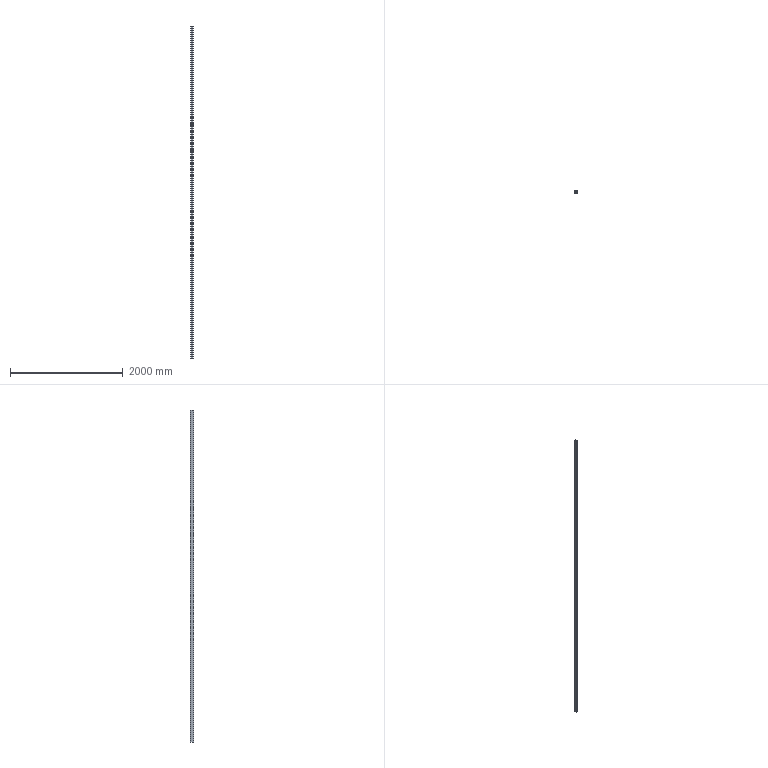Part | SolidWorks | features Extrusion 1 | 1 solid | 18 faces | box 40 x 60 x 5880 mm | volume 2698361 mm3 | plane 10 | cylinder 8 | commonest cylinder face diameters 5 x4 10 x4
STEP:
#1=CARTESIAN_POINT('',(35.,0.,5880.));
#2=VERTEX_POINT('',#1);
#3=CARTESIAN_POINT('',(40.,5.,5880.));
#4=VERTEX_POINT('',#3);
#5=CARTESIAN_POINT('',(35.,5.,5880.));
#6=DIRECTION('',(0.,0.,1.));
#7=DIRECTION('',(-1.,0.,0.));
#8=AXIS2_PLACEMENT_3D('',#5,#6,#7);
#9=CIRCLE('',#8,5.);
#10=EDGE_CURVE('',#2,#4,#9,.T.);
#11=ORIENTED_EDGE('',*,*,#10,.T.);
#12=CARTESIAN_POINT('',(40.,55.,5880.));
#13=VERTEX_POINT('',#12);
#14=CARTESIAN_POINT('',(40.,5.,5880.));
#15=DIRECTION('',(0.,1.,0.));
#16=VECTOR('',#15,1000.);
#17=LINE('',#14,#16);
#18=EDGE_CURVE('',#4,#13,#17,.T.);
#19=ORIENTED_EDGE('',*,*,#18,.T.);
#20=CARTESIAN_POINT('',(35.,60.,5880.));
#21=VERTEX_POINT('',#20);
#22=CARTESIAN_POINT('',(35.,55.,5880.));
#23=DIRECTION('',(0.,0.,1.));
#24=DIRECTION('',(1.,0.,0.));
#25=AXIS2_PLACEMENT_3D('',#22,#23,#24);
#26=CIRCLE('',#25,5.);
#27=EDGE_CURVE('',#13,#21,#26,.T.);
#28=ORIENTED_EDGE('',*,*,#27,.T.);
#29=CARTESIAN_POINT('',(5.,60.,5880.));
#30=VERTEX_POINT('',#29);
#31=CARTESIAN_POINT('',(5.,60.,5880.));
#32=DIRECTION('',(-1.,0.,0.));
#33=VECTOR('',#32,1000.);
#34=LINE('',#31,#33);
#35=EDGE_CURVE('',#21,#30,#34,.T.);
#36=ORIENTED_EDGE('',*,*,#35,.T.);
#37=CARTESIAN_POINT('',(0.,55.,5880.));
#38=VERTEX_POINT('',#37);
#39=CARTESIAN_POINT('',(5.,55.,5880.));
#40=DIRECTION('',(0.,0.,1.));
#41=DIRECTION('',(-1.,0.,0.));
#42=AXIS2_PLACEMENT_3D('',#39,#40,#41);
#43=CIRCLE('',#42,5.);
#44=EDGE_CURVE('',#30,#38,#43,.T.);
#45=ORIENTED_EDGE('',*,*,#44,.T.);
#46=CARTESIAN_POINT('',(0.,5.,5880.));
#47=VERTEX_POINT('',#46);
#48=CARTESIAN_POINT('',(0.,5.,5880.));
#49=DIRECTION('',(0.,-1.,0.));
#50=VECTOR('',#49,1000.);
#51=LINE('',#48,#50);
#52=EDGE_CURVE('',#38,#47,#51,.T.);
#53=ORIENTED_EDGE('',*,*,#52,.T.);
#54=CARTESIAN_POINT('',(5.,0.,5880.));
#55=VERTEX_POINT('',#54);
#56=CARTESIAN_POINT('',(5.,5.,5880.));
#57=DIRECTION('',(0.,0.,1.));
#58=DIRECTION('',(-1.,0.,0.));
#59=AXIS2_PLACEMENT_3D('',#56,#57,#58);
#60=CIRCLE('',#59,5.);
#61=EDGE_CURVE('',#47,#55,#60,.T.);
#62=ORIENTED_EDGE('',*,*,#61,.T.);
#63=CARTESIAN_POINT('',(5.,0.,5880.));
#64=DIRECTION('',(1.,0.,0.));
#65=VECTOR('',#64,1000.);
#66=LINE('',#63,#65);
#67=EDGE_CURVE('',#55,#2,#66,.T.);
#68=ORIENTED_EDGE('',*,*,#67,.T.);
#69=EDGE_LOOP('',(#11,#19,#28,#36,#45,#53,#62,#68));
#70=FACE_OUTER_BOUND('',#69,.T.);
#71=CARTESIAN_POINT('',(2.5,5.,5880.));
#72=VERTEX_POINT('',#71);
#73=CARTESIAN_POINT('',(5.,2.5,5880.));
#74=VERTEX_POINT('',#73);
#75=CARTESIAN_POINT('',(5.,5.,5880.));
#76=DIRECTION('',(0.,0.,1.));
#77=DIRECTION('',(-1.,0.,0.));
#78=AXIS2_PLACEMENT_3D('',#75,#76,#77);
#79=CIRCLE('',#78,2.5);
#80=EDGE_CURVE('',#72,#74,#79,.T.);
#81=ORIENTED_EDGE('',*,*,#80,.F.);
#82=CARTESIAN_POINT('',(2.5,55.,5880.));
#83=VERTEX_POINT('',#82);
#84=CARTESIAN_POINT('',(2.5,5.,5880.));
#85=DIRECTION('',(0.,-1.,0.));
#86=VECTOR('',#85,1000.);
#87=LINE('',#84,#86);
#88=EDGE_CURVE('',#83,#72,#87,.T.);
#89=ORIENTED_EDGE('',*,*,#88,.F.);
#90=CARTESIAN_POINT('',(5.,57.5,5880.));
#91=VERTEX_POINT('',#90);
#92=CARTESIAN_POINT('',(5.,55.,5880.));
#93=DIRECTION('',(0.,0.,1.));
#94=DIRECTION('',(-1.,0.,0.));
#95=AXIS2_PLACEMENT_3D('',#92,#93,#94);
#96=CIRCLE('',#95,2.5);
#97=EDGE_CURVE('',#91,#83,#96,.T.);
#98=ORIENTED_EDGE('',*,*,#97,.F.);
#99=CARTESIAN_POINT('',(35.,57.5,5880.));
#100=VERTEX_POINT('',#99);
#101=CARTESIAN_POINT('',(5.,57.5,5880.));
#102=DIRECTION('',(-1.,0.,0.));
#103=VECTOR('',#102,1000.);
#104=LINE('',#101,#103);
#105=EDGE_CURVE('',#100,#91,#104,.T.);
#106=ORIENTED_EDGE('',*,*,#105,.F.);
#107=CARTESIAN_POINT('',(37.5,55.,5880.));
#108=VERTEX_POINT('',#107);
#109=CARTESIAN_POINT('',(35.,55.,5880.));
#110=DIRECTION('',(0.,0.,1.));
#111=DIRECTION('',(1.,0.,0.));
#112=AXIS2_PLACEMENT_3D('',#109,#110,#111);
#113=CIRCLE('',#112,2.5);
#114=EDGE_CURVE('',#108,#100,#113,.T.);
#115=ORIENTED_EDGE('',*,*,#114,.F.);
#116=CARTESIAN_POINT('',(37.5,5.,5880.));
#117=VERTEX_POINT('',#116);
#118=CARTESIAN_POINT('',(37.5,5.,5880.));
#119=DIRECTION('',(0.,1.,0.));
#120=VECTOR('',#119,1000.);
#121=LINE('',#118,#120);
#122=EDGE_CURVE('',#117,#108,#121,.T.);
#123=ORIENTED_EDGE('',*,*,#122,.F.);
#124=CARTESIAN_POINT('',(35.,2.5,5880.));
#125=VERTEX_POINT('',#124);
#126=CARTESIAN_POINT('',(35.,5.,5880.));
#127=DIRECTION('',(0.,0.,1.));
#128=DIRECTION('',(-1.,0.,0.));
#129=AXIS2_PLACEMENT_3D('',#126,#127,#128);
#130=CIRCLE('',#129,2.5);
#131=EDGE_CURVE('',#125,#117,#130,.T.);
#132=ORIENTED_EDGE('',*,*,#131,.F.);
#133=CARTESIAN_POINT('',(5.,2.5,5880.));
#134=DIRECTION('',(1.,0.,0.));
#135=VECTOR('',#134,1000.);
#136=LINE('',#133,#135);
#137=EDGE_CURVE('',#74,#125,#136,.T.);
#138=ORIENTED_EDGE('',*,*,#137,.F.);
#139=EDGE_LOOP('',(#81,#89,#98,#106,#115,#123,#132,#138));
#140=FACE_BOUND('',#139,.T.);
#141=CARTESIAN_POINT('',(35.,5.,5880.));
#142=DIRECTION('',(0.,0.,-1.));
#143=DIRECTION('',(-1.,0.,0.));
#144=AXIS2_PLACEMENT_3D('',#141,#142,#143);
#145=PLANE('',#144);
#146=ADVANCED_FACE('',(#70,#140),#145,.F.);
#147=CARTESIAN_POINT('',(35.,0.,0.));
#148=VERTEX_POINT('',#147);
#149=CARTESIAN_POINT('',(40.,5.,0.));
#150=VERTEX_POINT('',#149);
#151=CARTESIAN_POINT('',(35.,5.,0.));
#152=DIRECTION('',(0.,0.,1.));
#153=DIRECTION('',(-1.,0.,0.));
#154=AXIS2_PLACEMENT_3D('',#151,#152,#153);
#155=CIRCLE('',#154,5.);
#156=EDGE_CURVE('',#148,#150,#155,.T.);
#157=ORIENTED_EDGE('',*,*,#156,.F.);
#158=CARTESIAN_POINT('',(5.,0.,0.));
#159=VERTEX_POINT('',#158);
#160=CARTESIAN_POINT('',(5.,0.,0.));
#161=DIRECTION('',(1.,0.,0.));
#162=VECTOR('',#161,1000.);
#163=LINE('',#160,#162);
#164=EDGE_CURVE('',#159,#148,#163,.T.);
#165=ORIENTED_EDGE('',*,*,#164,.F.);
#166=CARTESIAN_POINT('',(0.,5.,0.));
#167=VERTEX_POINT('',#166);
#168=CARTESIAN_POINT('',(5.,5.,0.));
#169=DIRECTION('',(0.,0.,1.));
#170=DIRECTION('',(-1.,0.,0.));
#171=AXIS2_PLACEMENT_3D('',#168,#169,#170);
#172=CIRCLE('',#171,5.);
#173=EDGE_CURVE('',#167,#159,#172,.T.);
#174=ORIENTED_EDGE('',*,*,#173,.F.);
#175=CARTESIAN_POINT('',(0.,55.,0.));
#176=VERTEX_POINT('',#175);
#177=CARTESIAN_POINT('',(0.,5.,0.));
#178=DIRECTION('',(0.,-1.,0.));
#179=VECTOR('',#178,1000.);
#180=LINE('',#177,#179);
#181=EDGE_CURVE('',#176,#167,#180,.T.);
#182=ORIENTED_EDGE('',*,*,#181,.F.);
#183=CARTESIAN_POINT('',(5.,60.,0.));
#184=VERTEX_POINT('',#183);
#185=CARTESIAN_POINT('',(5.,55.,0.));
#186=DIRECTION('',(0.,0.,1.));
#187=DIRECTION('',(-1.,0.,0.));
#188=AXIS2_PLACEMENT_3D('',#185,#186,#187);
#189=CIRCLE('',#188,5.);
#190=EDGE_CURVE('',#184,#176,#189,.T.);
#191=ORIENTED_EDGE('',*,*,#190,.F.);
#192=CARTESIAN_POINT('',(35.,60.,0.));
#193=VERTEX_POINT('',#192);
#194=CARTESIAN_POINT('',(5.,60.,0.));
#195=DIRECTION('',(-1.,0.,0.));
#196=VECTOR('',#195,1000.);
#197=LINE('',#194,#196);
#198=EDGE_CURVE('',#193,#184,#197,.T.);
#199=ORIENTED_EDGE('',*,*,#198,.F.);
#200=CARTESIAN_POINT('',(40.,55.,0.));
#201=VERTEX_POINT('',#200);
#202=CARTESIAN_POINT('',(35.,55.,0.));
#203=DIRECTION('',(0.,0.,1.));
#204=DIRECTION('',(1.,0.,0.));
#205=AXIS2_PLACEMENT_3D('',#202,#203,#204);
#206=CIRCLE('',#205,5.);
#207=EDGE_CURVE('',#201,#193,#206,.T.);
#208=ORIENTED_EDGE('',*,*,#207,.F.);
#209=CARTESIAN_POINT('',(40.,5.,0.));
#210=DIRECTION('',(0.,1.,0.));
#211=VECTOR('',#210,1000.);
#212=LINE('',#209,#211);
#213=EDGE_CURVE('',#150,#201,#212,.T.);
#214=ORIENTED_EDGE('',*,*,#213,.F.);
#215=EDGE_LOOP('',(#157,#165,#174,#182,#191,#199,#208,#214));
#216=FACE_OUTER_BOUND('',#215,.T.);
#217=CARTESIAN_POINT('',(2.5,55.,0.));
#218=VERTEX_POINT('',#217);
#219=CARTESIAN_POINT('',(2.5,5.,0.));
#220=VERTEX_POINT('',#219);
#221=CARTESIAN_POINT('',(2.5,5.,0.));
#222=DIRECTION('',(0.,-1.,0.));
#223=VECTOR('',#222,1000.);
#224=LINE('',#221,#223);
#225=EDGE_CURVE('',#218,#220,#224,.T.);
#226=ORIENTED_EDGE('',*,*,#225,.T.);
#227=CARTESIAN_POINT('',(5.,2.5,0.));
#228=VERTEX_POINT('',#227);
#229=CARTESIAN_POINT('',(5.,5.,0.));
#230=DIRECTION('',(0.,0.,1.));
#231=DIRECTION('',(-1.,0.,0.));
#232=AXIS2_PLACEMENT_3D('',#229,#230,#231);
#233=CIRCLE('',#232,2.5);
#234=EDGE_CURVE('',#220,#228,#233,.T.);
#235=ORIENTED_EDGE('',*,*,#234,.T.);
#236=CARTESIAN_POINT('',(35.,2.5,0.));
#237=VERTEX_POINT('',#236);
#238=CARTESIAN_POINT('',(5.,2.5,0.));
#239=DIRECTION('',(1.,0.,0.));
#240=VECTOR('',#239,1000.);
#241=LINE('',#238,#240);
#242=EDGE_CURVE('',#228,#237,#241,.T.);
#243=ORIENTED_EDGE('',*,*,#242,.T.);
#244=CARTESIAN_POINT('',(37.5,5.,0.));
#245=VERTEX_POINT('',#244);
#246=CARTESIAN_POINT('',(35.,5.,0.));
#247=DIRECTION('',(0.,0.,1.));
#248=DIRECTION('',(-1.,0.,0.));
#249=AXIS2_PLACEMENT_3D('',#246,#247,#248);
#250=CIRCLE('',#249,2.5);
#251=EDGE_CURVE('',#237,#245,#250,.T.);
#252=ORIENTED_EDGE('',*,*,#251,.T.);
#253=CARTESIAN_POINT('',(37.5,55.,0.));
#254=VERTEX_POINT('',#253);
#255=CARTESIAN_POINT('',(37.5,5.,0.));
#256=DIRECTION('',(0.,1.,0.));
#257=VECTOR('',#256,1000.);
#258=LINE('',#255,#257);
#259=EDGE_CURVE('',#245,#254,#258,.T.);
#260=ORIENTED_EDGE('',*,*,#259,.T.);
#261=CARTESIAN_POINT('',(35.,57.5,0.));
#262=VERTEX_POINT('',#261);
#263=CARTESIAN_POINT('',(35.,55.,0.));
#264=DIRECTION('',(0.,0.,1.));
#265=DIRECTION('',(1.,0.,0.));
#266=AXIS2_PLACEMENT_3D('',#263,#264,#265);
#267=CIRCLE('',#266,2.5);
#268=EDGE_CURVE('',#254,#262,#267,.T.);
#269=ORIENTED_EDGE('',*,*,#268,.T.);
#270=CARTESIAN_POINT('',(5.,57.5,0.));
#271=VERTEX_POINT('',#270);
#272=CARTESIAN_POINT('',(5.,57.5,0.));
#273=DIRECTION('',(-1.,0.,0.));
#274=VECTOR('',#273,1000.);
#275=LINE('',#272,#274);
#276=EDGE_CURVE('',#262,#271,#275,.T.);
#277=ORIENTED_EDGE('',*,*,#276,.T.);
#278=CARTESIAN_POINT('',(5.,55.,0.));
#279=DIRECTION('',(0.,0.,1.));
#280=DIRECTION('',(-1.,0.,0.));
#281=AXIS2_PLACEMENT_3D('',#278,#279,#280);
#282=CIRCLE('',#281,2.5);
#283=EDGE_CURVE('',#271,#218,#282,.T.);
#284=ORIENTED_EDGE('',*,*,#283,.T.);
#285=EDGE_LOOP('',(#226,#235,#243,#252,#260,#269,#277,#284));
#286=FACE_BOUND('',#285,.T.);
#287=CARTESIAN_POINT('',(35.,5.,0.));
#288=DIRECTION('',(0.,0.,-1.));
#289=DIRECTION('',(-1.,0.,0.));
#290=AXIS2_PLACEMENT_3D('',#287,#288,#289);
#291=PLANE('',#290);
#292=ADVANCED_FACE('',(#216,#286),#291,.T.);
#293=ORIENTED_EDGE('',*,*,#156,.T.);
#294=CARTESIAN_POINT('',(40.,5.,5880.));
#295=DIRECTION('',(0.,0.,-1.));
#296=VECTOR('',#295,1000.);
#297=LINE('',#294,#296);
#298=EDGE_CURVE('',#4,#150,#297,.T.);
#299=ORIENTED_EDGE('',*,*,#298,.F.);
#300=ORIENTED_EDGE('',*,*,#10,.F.);
#301=CARTESIAN_POINT('',(35.,0.,5880.));
#302=DIRECTION('',(0.,0.,-1.));
#303=VECTOR('',#302,1000.);
#304=LINE('',#301,#303);
#305=EDGE_CURVE('',#2,#148,#304,.T.);
#306=ORIENTED_EDGE('',*,*,#305,.T.);
#307=EDGE_LOOP('',(#293,#299,#300,#306));
#308=FACE_OUTER_BOUND('',#307,.T.);
#309=CARTESIAN_POINT('',(35.,5.,5880.));
#310=DIRECTION('',(0.,0.,-1.));
#311=DIRECTION('',(-1.,0.,0.));
#312=AXIS2_PLACEMENT_3D('',#309,#310,#311);
#313=CYLINDRICAL_SURFACE('',#312,5.);
#314=ADVANCED_FACE('',(#308),#313,.T.);
#315=ORIENTED_EDGE('',*,*,#213,.T.);
#316=CARTESIAN_POINT('',(40.,55.,5880.));
#317=DIRECTION('',(0.,0.,-1.));
#318=VECTOR('',#317,1000.);
#319=LINE('',#316,#318);
#320=EDGE_CURVE('',#13,#201,#319,.T.);
#321=ORIENTED_EDGE('',*,*,#320,.F.);
#322=ORIENTED_EDGE('',*,*,#18,.F.);
#323=ORIENTED_EDGE('',*,*,#298,.T.);
#324=EDGE_LOOP('',(#315,#321,#322,#323));
#325=FACE_OUTER_BOUND('',#324,.T.);
#326=CARTESIAN_POINT('',(40.,5.,5880.));
#327=DIRECTION('',(-1.,0.,0.));
#328=DIRECTION('',(0.,-1.,0.));
#329=AXIS2_PLACEMENT_3D('',#326,#327,#328);
#330=PLANE('',#329);
#331=ADVANCED_FACE('',(#325),#330,.F.);
#332=ORIENTED_EDGE('',*,*,#207,.T.);
#333=CARTESIAN_POINT('',(35.,60.,5880.));
#334=DIRECTION('',(0.,0.,-1.));
#335=VECTOR('',#334,1000.);
#336=LINE('',#333,#335);
#337=EDGE_CURVE('',#21,#193,#336,.T.);
#338=ORIENTED_EDGE('',*,*,#337,.F.);
#339=ORIENTED_EDGE('',*,*,#27,.F.);
#340=ORIENTED_EDGE('',*,*,#320,.T.);
#341=EDGE_LOOP('',(#332,#338,#339,#340));
#342=FACE_OUTER_BOUND('',#341,.T.);
#343=CARTESIAN_POINT('',(35.,55.,5880.));
#344=DIRECTION('',(0.,0.,-1.));
#345=DIRECTION('',(-1.,0.,0.));
#346=AXIS2_PLACEMENT_3D('',#343,#344,#345);
#347=CYLINDRICAL_SURFACE('',#346,5.);
#348=ADVANCED_FACE('',(#342),#347,.T.);
#349=ORIENTED_EDGE('',*,*,#198,.T.);
#350=CARTESIAN_POINT('',(5.,60.,5880.));
#351=DIRECTION('',(0.,0.,-1.));
#352=VECTOR('',#351,1000.);
#353=LINE('',#350,#352);
#354=EDGE_CURVE('',#30,#184,#353,.T.);
#355=ORIENTED_EDGE('',*,*,#354,.F.);
#356=ORIENTED_EDGE('',*,*,#35,.F.);
#357=ORIENTED_EDGE('',*,*,#337,.T.);
#358=EDGE_LOOP('',(#349,#355,#356,#357));
#359=FACE_OUTER_BOUND('',#358,.T.);
#360=CARTESIAN_POINT('',(5.,60.,5880.));
#361=DIRECTION('',(0.,-1.,0.));
#362=DIRECTION('',(0.,0.,-1.));
#363=AXIS2_PLACEMENT_3D('',#360,#361,#362);
#364=PLANE('',#363);
#365=ADVANCED_FACE('',(#359),#364,.F.);
#366=ORIENTED_EDGE('',*,*,#190,.T.);
#367=CARTESIAN_POINT('',(0.,55.,5880.));
#368=DIRECTION('',(0.,0.,-1.));
#369=VECTOR('',#368,1000.);
#370=LINE('',#367,#369);
#371=EDGE_CURVE('',#38,#176,#370,.T.);
#372=ORIENTED_EDGE('',*,*,#371,.F.);
#373=ORIENTED_EDGE('',*,*,#44,.F.);
#374=ORIENTED_EDGE('',*,*,#354,.T.);
#375=EDGE_LOOP('',(#366,#372,#373,#374));
#376=FACE_OUTER_BOUND('',#375,.T.);
#377=CARTESIAN_POINT('',(5.,55.,5880.));
#378=DIRECTION('',(0.,0.,-1.));
#379=DIRECTION('',(-1.,0.,0.));
#380=AXIS2_PLACEMENT_3D('',#377,#378,#379);
#381=CYLINDRICAL_SURFACE('',#380,5.);
#382=ADVANCED_FACE('',(#376),#381,.T.);
#383=ORIENTED_EDGE('',*,*,#181,.T.);
#384=CARTESIAN_POINT('',(0.,5.,5880.));
#385=DIRECTION('',(0.,0.,-1.));
#386=VECTOR('',#385,1000.);
#387=LINE('',#384,#386);
#388=EDGE_CURVE('',#47,#167,#387,.T.);
#389=ORIENTED_EDGE('',*,*,#388,.F.);
#390=ORIENTED_EDGE('',*,*,#52,.F.);
#391=ORIENTED_EDGE('',*,*,#371,.T.);
#392=EDGE_LOOP('',(#383,#389,#390,#391));
#393=FACE_OUTER_BOUND('',#392,.T.);
#394=CARTESIAN_POINT('',(0.,5.,5880.));
#395=DIRECTION('',(1.,0.,0.));
#396=DIRECTION('',(0.,1.,0.));
#397=AXIS2_PLACEMENT_3D('',#394,#395,#396);
#398=PLANE('',#397);
#399=ADVANCED_FACE('',(#393),#398,.F.);
#400=ORIENTED_EDGE('',*,*,#173,.T.);
#401=CARTESIAN_POINT('',(5.,0.,5880.));
#402=DIRECTION('',(0.,0.,-1.));
#403=VECTOR('',#402,1000.);
#404=LINE('',#401,#403);
#405=EDGE_CURVE('',#55,#159,#404,.T.);
#406=ORIENTED_EDGE('',*,*,#405,.F.);
#407=ORIENTED_EDGE('',*,*,#61,.F.);
#408=ORIENTED_EDGE('',*,*,#388,.T.);
#409=EDGE_LOOP('',(#400,#406,#407,#408));
#410=FACE_OUTER_BOUND('',#409,.T.);
#411=CARTESIAN_POINT('',(5.,5.,5880.));
#412=DIRECTION('',(0.,0.,-1.));
#413=DIRECTION('',(-1.,0.,0.));
#414=AXIS2_PLACEMENT_3D('',#411,#412,#413);
#415=CYLINDRICAL_SURFACE('',#414,5.);
#416=ADVANCED_FACE('',(#410),#415,.T.);
#417=ORIENTED_EDGE('',*,*,#164,.T.);
#418=ORIENTED_EDGE('',*,*,#305,.F.);
#419=ORIENTED_EDGE('',*,*,#67,.F.);
#420=ORIENTED_EDGE('',*,*,#405,.T.);
#421=EDGE_LOOP('',(#417,#418,#419,#420));
#422=FACE_OUTER_BOUND('',#421,.T.);
#423=CARTESIAN_POINT('',(5.,0.,5880.));
#424=DIRECTION('',(0.,1.,0.));
#425=DIRECTION('',(0.,0.,1.));
#426=AXIS2_PLACEMENT_3D('',#423,#424,#425);
#427=PLANE('',#426);
#428=ADVANCED_FACE('',(#422),#427,.F.);
#429=ORIENTED_EDGE('',*,*,#234,.F.);
#430=CARTESIAN_POINT('',(2.5,5.,5880.));
#431=DIRECTION('',(0.,0.,-1.));
#432=VECTOR('',#431,1000.);
#433=LINE('',#430,#432);
#434=EDGE_CURVE('',#72,#220,#433,.T.);
#435=ORIENTED_EDGE('',*,*,#434,.F.);
#436=ORIENTED_EDGE('',*,*,#80,.T.);
#437=CARTESIAN_POINT('',(5.,2.5,5880.));
#438=DIRECTION('',(0.,0.,-1.));
#439=VECTOR('',#438,1000.);
#440=LINE('',#437,#439);
#441=EDGE_CURVE('',#74,#228,#440,.T.);
#442=ORIENTED_EDGE('',*,*,#441,.T.);
#443=EDGE_LOOP('',(#429,#435,#436,#442));
#444=FACE_OUTER_BOUND('',#443,.T.);
#445=CARTESIAN_POINT('',(5.,5.,5880.));
#446=DIRECTION('',(0.,0.,-1.));
#447=DIRECTION('',(-1.,0.,0.));
#448=AXIS2_PLACEMENT_3D('',#445,#446,#447);
#449=CYLINDRICAL_SURFACE('',#448,2.5);
#450=ADVANCED_FACE('',(#444),#449,.F.);
#451=ORIENTED_EDGE('',*,*,#242,.F.);
#452=ORIENTED_EDGE('',*,*,#441,.F.);
#453=ORIENTED_EDGE('',*,*,#137,.T.);
#454=CARTESIAN_POINT('',(35.,2.5,5880.));
#455=DIRECTION('',(0.,0.,-1.));
#456=VECTOR('',#455,1000.);
#457=LINE('',#454,#456);
#458=EDGE_CURVE('',#125,#237,#457,.T.);
#459=ORIENTED_EDGE('',*,*,#458,.T.);
#460=EDGE_LOOP('',(#451,#452,#453,#459));
#461=FACE_OUTER_BOUND('',#460,.T.);
#462=CARTESIAN_POINT('',(5.,2.5,5880.));
#463=DIRECTION('',(0.,1.,0.));
#464=DIRECTION('',(0.,0.,1.));
#465=AXIS2_PLACEMENT_3D('',#462,#463,#464);
#466=PLANE('',#465);
#467=ADVANCED_FACE('',(#461),#466,.T.);
#468=ORIENTED_EDGE('',*,*,#251,.F.);
#469=ORIENTED_EDGE('',*,*,#458,.F.);
#470=ORIENTED_EDGE('',*,*,#131,.T.);
#471=CARTESIAN_POINT('',(37.5,5.,5880.));
#472=DIRECTION('',(0.,0.,-1.));
#473=VECTOR('',#472,1000.);
#474=LINE('',#471,#473);
#475=EDGE_CURVE('',#117,#245,#474,.T.);
#476=ORIENTED_EDGE('',*,*,#475,.T.);
#477=EDGE_LOOP('',(#468,#469,#470,#476));
#478=FACE_OUTER_BOUND('',#477,.T.);
#479=CARTESIAN_POINT('',(35.,5.,5880.));
#480=DIRECTION('',(0.,0.,-1.));
#481=DIRECTION('',(-1.,0.,0.));
#482=AXIS2_PLACEMENT_3D('',#479,#480,#481);
#483=CYLINDRICAL_SURFACE('',#482,2.5);
#484=ADVANCED_FACE('',(#478),#483,.F.);
#485=ORIENTED_EDGE('',*,*,#259,.F.);
#486=ORIENTED_EDGE('',*,*,#475,.F.);
#487=ORIENTED_EDGE('',*,*,#122,.T.);
#488=CARTESIAN_POINT('',(37.5,55.,5880.));
#489=DIRECTION('',(0.,0.,-1.));
#490=VECTOR('',#489,1000.);
#491=LINE('',#488,#490);
#492=EDGE_CURVE('',#108,#254,#491,.T.);
#493=ORIENTED_EDGE('',*,*,#492,.T.);
#494=EDGE_LOOP('',(#485,#486,#487,#493));
#495=FACE_OUTER_BOUND('',#494,.T.);
#496=CARTESIAN_POINT('',(37.5,5.,5880.));
#497=DIRECTION('',(-1.,0.,0.));
#498=DIRECTION('',(0.,0.,1.));
#499=AXIS2_PLACEMENT_3D('',#496,#497,#498);
#500=PLANE('',#499);
#501=ADVANCED_FACE('',(#495),#500,.T.);
#502=ORIENTED_EDGE('',*,*,#268,.F.);
#503=ORIENTED_EDGE('',*,*,#492,.F.);
#504=ORIENTED_EDGE('',*,*,#114,.T.);
#505=CARTESIAN_POINT('',(35.,57.5,5880.));
#506=DIRECTION('',(0.,0.,-1.));
#507=VECTOR('',#506,1000.);
#508=LINE('',#505,#507);
#509=EDGE_CURVE('',#100,#262,#508,.T.);
#510=ORIENTED_EDGE('',*,*,#509,.T.);
#511=EDGE_LOOP('',(#502,#503,#504,#510));
#512=FACE_OUTER_BOUND('',#511,.T.);
#513=CARTESIAN_POINT('',(35.,55.,5880.));
#514=DIRECTION('',(0.,0.,-1.));
#515=DIRECTION('',(-1.,0.,0.));
#516=AXIS2_PLACEMENT_3D('',#513,#514,#515);
#517=CYLINDRICAL_SURFACE('',#516,2.5);
#518=ADVANCED_FACE('',(#512),#517,.F.);
#519=ORIENTED_EDGE('',*,*,#276,.F.);
#520=ORIENTED_EDGE('',*,*,#509,.F.);
#521=ORIENTED_EDGE('',*,*,#105,.T.);
#522=CARTESIAN_POINT('',(5.,57.5,5880.));
#523=DIRECTION('',(0.,0.,-1.));
#524=VECTOR('',#523,1000.);
#525=LINE('',#522,#524);
#526=EDGE_CURVE('',#91,#271,#525,.T.);
#527=ORIENTED_EDGE('',*,*,#526,.T.);
#528=EDGE_LOOP('',(#519,#520,#521,#527));
#529=FACE_OUTER_BOUND('',#528,.T.);
#530=CARTESIAN_POINT('',(5.,57.5,5880.));
#531=DIRECTION('',(0.,-1.,0.));
#532=DIRECTION('',(1.,0.,0.));
#533=AXIS2_PLACEMENT_3D('',#530,#531,#532);
#534=PLANE('',#533);
#535=ADVANCED_FACE('',(#529),#534,.T.);
#536=ORIENTED_EDGE('',*,*,#283,.F.);
#537=ORIENTED_EDGE('',*,*,#526,.F.);
#538=ORIENTED_EDGE('',*,*,#97,.T.);
#539=CARTESIAN_POINT('',(2.5,55.,5880.));
#540=DIRECTION('',(0.,0.,-1.));
#541=VECTOR('',#540,1000.);
#542=LINE('',#539,#541);
#543=EDGE_CURVE('',#83,#218,#542,.T.);
#544=ORIENTED_EDGE('',*,*,#543,.T.);
#545=EDGE_LOOP('',(#536,#537,#538,#544));
#546=FACE_OUTER_BOUND('',#545,.T.);
#547=CARTESIAN_POINT('',(5.,55.,5880.));
#548=DIRECTION('',(0.,0.,-1.));
#549=DIRECTION('',(-1.,0.,0.));
#550=AXIS2_PLACEMENT_3D('',#547,#548,#549);
#551=CYLINDRICAL_SURFACE('',#550,2.5);
#552=ADVANCED_FACE('',(#546),#551,.F.);
#553=ORIENTED_EDGE('',*,*,#225,.F.);
#554=ORIENTED_EDGE('',*,*,#543,.F.);
#555=ORIENTED_EDGE('',*,*,#88,.T.);
#556=ORIENTED_EDGE('',*,*,#434,.T.);
#557=EDGE_LOOP('',(#553,#554,#555,#556));
#558=FACE_OUTER_BOUND('',#557,.T.);
#559=CARTESIAN_POINT('',(2.5,5.,5880.));
#560=DIRECTION('',(1.,0.,0.));
#561=DIRECTION('',(0.,0.,-1.));
#562=AXIS2_PLACEMENT_3D('',#559,#560,#561);
#563=PLANE('',#562);
#564=ADVANCED_FACE('',(#558),#563,.T.);
#565=CLOSED_SHELL('',(#146,#292,#314,#331,#348,#365,#382,#399,#416,#428,#450,#467,#484,#501,#518,#535,#552,#564));
#566=MANIFOLD_SOLID_BREP('',#565);
#567=CARTESIAN_POINT('',(0.,0.,0.));
#568=DIRECTION('',(0.,0.,1.));
#569=DIRECTION('',(1.,0.,0.));
#570=AXIS2_PLACEMENT_3D('',#567,#568,#569);
#571=(LENGTH_UNIT()NAMED_UNIT(*)SI_UNIT(.MILLI.,.METRE.));
#572=UNCERTAINTY_MEASURE_WITH_UNIT(LENGTH_MEASURE(0.00001),#571,'','');
#573=(NAMED_UNIT(*)PLANE_ANGLE_UNIT()SI_UNIT($,.RADIAN.));
#574=(NAMED_UNIT(*)SI_UNIT($,.STERADIAN.)SOLID_ANGLE_UNIT());
#575=(GEOMETRIC_REPRESENTATION_CONTEXT(3)GLOBAL_UNCERTAINTY_ASSIGNED_CONTEXT((#572))GLOBAL_UNIT_ASSIGNED_CONTEXT((#571,#573,#574))REPRESENTATION_CONTEXT('',''));
#576=ADVANCED_BREP_SHAPE_REPRESENTATION('',(#566,#570),#575);